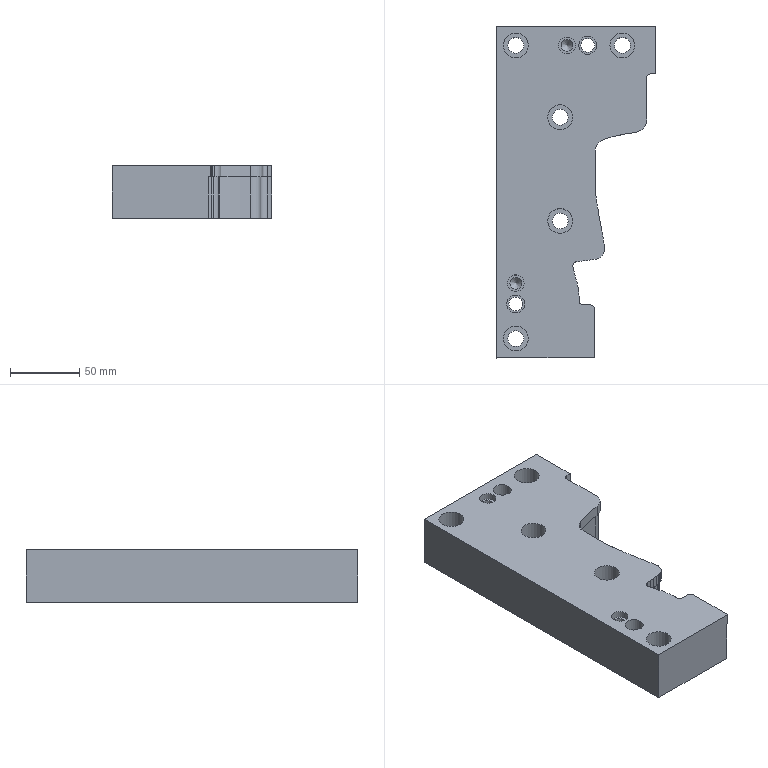Part | STEP file | lll_id4678_x_t | 1 solid | 132 faces | box 115 x 240 x 38 mm | volume 703311 mm3 | cylinder 102 | plane 28 | cone 2 | commonest cylinder face diameters 11.509 x5 18.008 x5 6 x4 10 x3 13 x3 3 x2